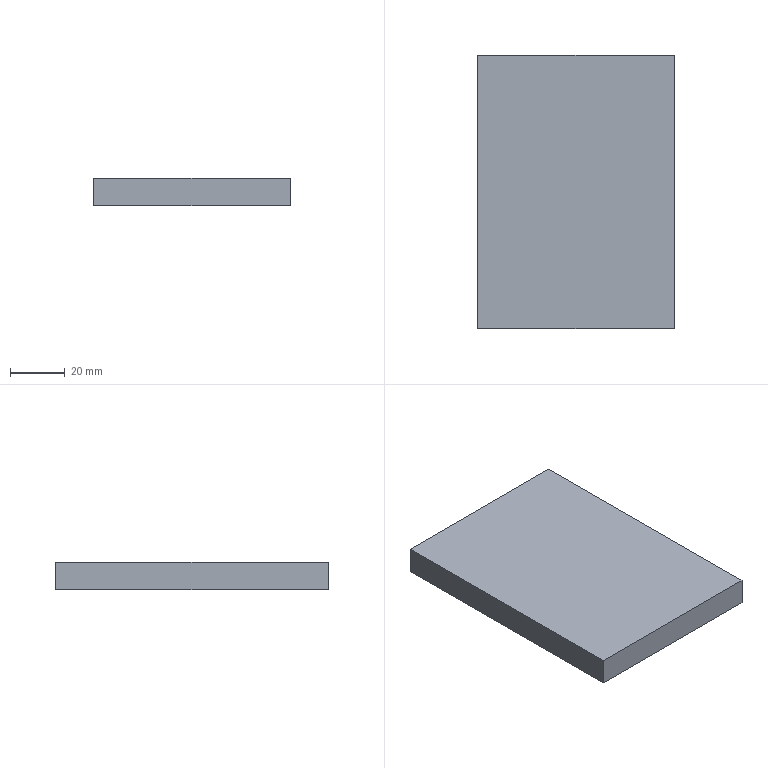Part | STEP file | Display 2 | 1 solid | 6 faces | box 72 x 100 x 10 mm | volume 72000 mm3 | plane 6
STEP:
#1=CARTESIAN_POINT('',(0.,0.,0.));
#2=DIRECTION('',(0.,0.,1.));
#3=DIRECTION('',(1.,0.,0.));
#4=AXIS2_PLACEMENT_3D('',#1,#2,#3);
#5=CARTESIAN_POINT('',(36.,-50.,10.));
#6=VERTEX_POINT('',#5);
#7=CARTESIAN_POINT('',(36.,50.,10.));
#8=VERTEX_POINT('',#7);
#9=CARTESIAN_POINT('',(36.,-50.,10.));
#10=DIRECTION('',(0.,1.,0.));
#11=VECTOR('',#10,1.);
#12=LINE('',#9,#11);
#13=CARTESIAN_POINT('',(-36.,-50.,10.));
#14=DIRECTION('',(0.,0.,1.));
#15=DIRECTION('',(1.,0.,0.));
#16=AXIS2_PLACEMENT_3D('',#13,#14,#15);
#17=PLANE('',#16);
#18=CARTESIAN_POINT('',(72.,0.));
#19=DIRECTION('',(0.,1.));
#20=VECTOR('',#19,1.);
#21=LINE('',#18,#20);
#22=(GEOMETRIC_REPRESENTATION_CONTEXT(2)PARAMETRIC_REPRESENTATION_CONTEXT()REPRESENTATION_CONTEXT('',''));
#23=DEFINITIONAL_REPRESENTATION('',(#21),#22);
#24=PCURVE('',#17,#23);
#25=CARTESIAN_POINT('',(36.,50.,10.));
#26=DIRECTION('',(-1.,0.,0.));
#27=DIRECTION('',(0.,-1.,0.));
#28=AXIS2_PLACEMENT_3D('',#25,#26,#27);
#29=PLANE('',#28);
#30=CARTESIAN_POINT('',(100.,0.));
#31=DIRECTION('',(-1.,0.));
#32=VECTOR('',#31,1.);
#33=LINE('',#30,#32);
#34=(GEOMETRIC_REPRESENTATION_CONTEXT(2)PARAMETRIC_REPRESENTATION_CONTEXT()REPRESENTATION_CONTEXT('',''));
#35=DEFINITIONAL_REPRESENTATION('',(#33),#34);
#36=PCURVE('',#29,#35);
#37=SURFACE_CURVE('',#12,(#24,#36),.PCURVE_S1.);
#38=EDGE_CURVE('',#6,#8,#37,.T.);
#39=ORIENTED_EDGE('',*,*,#38,.T.);
#40=CARTESIAN_POINT('',(-36.,50.,10.));
#41=VERTEX_POINT('',#40);
#42=CARTESIAN_POINT('',(-36.,50.,10.));
#43=DIRECTION('',(-1.,0.,0.));
#44=VECTOR('',#43,1.);
#45=LINE('',#42,#44);
#46=CARTESIAN_POINT('',(0.,100.));
#47=DIRECTION('',(-1.,0.));
#48=VECTOR('',#47,1.);
#49=LINE('',#46,#48);
#50=(GEOMETRIC_REPRESENTATION_CONTEXT(2)PARAMETRIC_REPRESENTATION_CONTEXT()REPRESENTATION_CONTEXT('',''));
#51=DEFINITIONAL_REPRESENTATION('',(#49),#50);
#52=PCURVE('',#17,#51);
#53=CARTESIAN_POINT('',(-36.,50.,10.));
#54=DIRECTION('',(0.,-1.,0.));
#55=DIRECTION('',(1.,0.,0.));
#56=AXIS2_PLACEMENT_3D('',#53,#54,#55);
#57=PLANE('',#56);
#58=CARTESIAN_POINT('',(0.,0.));
#59=DIRECTION('',(-1.,0.));
#60=VECTOR('',#59,1.);
#61=LINE('',#58,#60);
#62=(GEOMETRIC_REPRESENTATION_CONTEXT(2)PARAMETRIC_REPRESENTATION_CONTEXT()REPRESENTATION_CONTEXT('',''));
#63=DEFINITIONAL_REPRESENTATION('',(#61),#62);
#64=PCURVE('',#57,#63);
#65=SURFACE_CURVE('',#45,(#52,#64),.PCURVE_S1.);
#66=EDGE_CURVE('',#8,#41,#65,.T.);
#67=ORIENTED_EDGE('',*,*,#66,.T.);
#68=CARTESIAN_POINT('',(-36.,-50.,10.));
#69=VERTEX_POINT('',#68);
#70=CARTESIAN_POINT('',(-36.,-50.,10.));
#71=DIRECTION('',(0.,-1.,0.));
#72=VECTOR('',#71,1.);
#73=LINE('',#70,#72);
#74=CARTESIAN_POINT('',(0.,0.));
#75=DIRECTION('',(0.,-1.));
#76=VECTOR('',#75,1.);
#77=LINE('',#74,#76);
#78=(GEOMETRIC_REPRESENTATION_CONTEXT(2)PARAMETRIC_REPRESENTATION_CONTEXT()REPRESENTATION_CONTEXT('',''));
#79=DEFINITIONAL_REPRESENTATION('',(#77),#78);
#80=PCURVE('',#17,#79);
#81=CARTESIAN_POINT('',(-36.,50.,10.));
#82=DIRECTION('',(1.,0.,0.));
#83=DIRECTION('',(0.,0.,-1.));
#84=AXIS2_PLACEMENT_3D('',#81,#82,#83);
#85=PLANE('',#84);
#86=CARTESIAN_POINT('',(0.,-100.));
#87=DIRECTION('',(0.,-1.));
#88=VECTOR('',#87,1.);
#89=LINE('',#86,#88);
#90=(GEOMETRIC_REPRESENTATION_CONTEXT(2)PARAMETRIC_REPRESENTATION_CONTEXT()REPRESENTATION_CONTEXT('',''));
#91=DEFINITIONAL_REPRESENTATION('',(#89),#90);
#92=PCURVE('',#85,#91);
#93=SURFACE_CURVE('',#73,(#80,#92),.PCURVE_S1.);
#94=EDGE_CURVE('',#41,#69,#93,.T.);
#95=ORIENTED_EDGE('',*,*,#94,.T.);
#96=CARTESIAN_POINT('',(-36.,-50.,10.));
#97=DIRECTION('',(1.,0.,0.));
#98=VECTOR('',#97,1.);
#99=LINE('',#96,#98);
#100=CARTESIAN_POINT('',(0.,0.));
#101=DIRECTION('',(1.,0.));
#102=VECTOR('',#101,1.);
#103=LINE('',#100,#102);
#104=(GEOMETRIC_REPRESENTATION_CONTEXT(2)PARAMETRIC_REPRESENTATION_CONTEXT()REPRESENTATION_CONTEXT('',''));
#105=DEFINITIONAL_REPRESENTATION('',(#103),#104);
#106=PCURVE('',#17,#105);
#107=CARTESIAN_POINT('',(-36.,-50.,10.));
#108=DIRECTION('',(0.,1.,0.));
#109=DIRECTION('',(-1.,0.,0.));
#110=AXIS2_PLACEMENT_3D('',#107,#108,#109);
#111=PLANE('',#110);
#112=CARTESIAN_POINT('',(0.,0.));
#113=DIRECTION('',(-1.,0.));
#114=VECTOR('',#113,1.);
#115=LINE('',#112,#114);
#116=(GEOMETRIC_REPRESENTATION_CONTEXT(2)PARAMETRIC_REPRESENTATION_CONTEXT()REPRESENTATION_CONTEXT('',''));
#117=DEFINITIONAL_REPRESENTATION('',(#115),#116);
#118=PCURVE('',#111,#117);
#119=SURFACE_CURVE('',#99,(#106,#118),.PCURVE_S1.);
#120=EDGE_CURVE('',#69,#6,#119,.T.);
#121=ORIENTED_EDGE('',*,*,#120,.T.);
#122=EDGE_LOOP('',(#39,#67,#95,#121));
#123=FACE_BOUND('',#122,.T.);
#124=ADVANCED_FACE('',(#123),#17,.T.);
#125=CARTESIAN_POINT('',(-36.,50.,0.));
#126=VERTEX_POINT('',#125);
#127=CARTESIAN_POINT('',(-36.,50.,10.));
#128=DIRECTION('',(0.,0.,-1.));
#129=VECTOR('',#128,1.);
#130=LINE('',#127,#129);
#131=CARTESIAN_POINT('',(0.,0.));
#132=DIRECTION('',(0.,-1.));
#133=VECTOR('',#132,1.);
#134=LINE('',#131,#133);
#135=(GEOMETRIC_REPRESENTATION_CONTEXT(2)PARAMETRIC_REPRESENTATION_CONTEXT()REPRESENTATION_CONTEXT('',''));
#136=DEFINITIONAL_REPRESENTATION('',(#134),#135);
#137=PCURVE('',#57,#136);
#138=CARTESIAN_POINT('',(0.,0.));
#139=DIRECTION('',(1.,0.));
#140=VECTOR('',#139,1.);
#141=LINE('',#138,#140);
#142=(GEOMETRIC_REPRESENTATION_CONTEXT(2)PARAMETRIC_REPRESENTATION_CONTEXT()REPRESENTATION_CONTEXT('',''));
#143=DEFINITIONAL_REPRESENTATION('',(#141),#142);
#144=PCURVE('',#85,#143);
#145=SURFACE_CURVE('',#130,(#137,#144),.PCURVE_S1.);
#146=EDGE_CURVE('',#41,#126,#145,.T.);
#147=ORIENTED_EDGE('',*,*,#146,.F.);
#148=ORIENTED_EDGE('',*,*,#66,.F.);
#149=CARTESIAN_POINT('',(36.,50.,0.));
#150=VERTEX_POINT('',#149);
#151=CARTESIAN_POINT('',(36.,50.,10.));
#152=DIRECTION('',(0.,0.,1.));
#153=VECTOR('',#152,1.);
#154=LINE('',#151,#153);
#155=CARTESIAN_POINT('',(72.,0.));
#156=DIRECTION('',(0.,1.));
#157=VECTOR('',#156,1.);
#158=LINE('',#155,#157);
#159=(GEOMETRIC_REPRESENTATION_CONTEXT(2)PARAMETRIC_REPRESENTATION_CONTEXT()REPRESENTATION_CONTEXT('',''));
#160=DEFINITIONAL_REPRESENTATION('',(#158),#159);
#161=PCURVE('',#57,#160);
#162=CARTESIAN_POINT('',(0.,0.));
#163=DIRECTION('',(0.,1.));
#164=VECTOR('',#163,1.);
#165=LINE('',#162,#164);
#166=(GEOMETRIC_REPRESENTATION_CONTEXT(2)PARAMETRIC_REPRESENTATION_CONTEXT()REPRESENTATION_CONTEXT('',''));
#167=DEFINITIONAL_REPRESENTATION('',(#165),#166);
#168=PCURVE('',#29,#167);
#169=SURFACE_CURVE('',#154,(#161,#168),.PCURVE_S1.);
#170=EDGE_CURVE('',#150,#8,#169,.T.);
#171=ORIENTED_EDGE('',*,*,#170,.F.);
#172=CARTESIAN_POINT('',(-36.,50.,0.));
#173=DIRECTION('',(1.,0.,0.));
#174=VECTOR('',#173,1.);
#175=LINE('',#172,#174);
#176=CARTESIAN_POINT('',(0.,-10.));
#177=DIRECTION('',(1.,0.));
#178=VECTOR('',#177,1.);
#179=LINE('',#176,#178);
#180=(GEOMETRIC_REPRESENTATION_CONTEXT(2)PARAMETRIC_REPRESENTATION_CONTEXT()REPRESENTATION_CONTEXT('',''));
#181=DEFINITIONAL_REPRESENTATION('',(#179),#180);
#182=PCURVE('',#57,#181);
#183=CARTESIAN_POINT('',(-36.,-50.,0.));
#184=DIRECTION('',(0.,0.,1.));
#185=DIRECTION('',(1.,0.,0.));
#186=AXIS2_PLACEMENT_3D('',#183,#184,#185);
#187=PLANE('',#186);
#188=CARTESIAN_POINT('',(0.,100.));
#189=DIRECTION('',(1.,0.));
#190=VECTOR('',#189,1.);
#191=LINE('',#188,#190);
#192=(GEOMETRIC_REPRESENTATION_CONTEXT(2)PARAMETRIC_REPRESENTATION_CONTEXT()REPRESENTATION_CONTEXT('',''));
#193=DEFINITIONAL_REPRESENTATION('',(#191),#192);
#194=PCURVE('',#187,#193);
#195=SURFACE_CURVE('',#175,(#182,#194),.PCURVE_S1.);
#196=EDGE_CURVE('',#126,#150,#195,.T.);
#197=ORIENTED_EDGE('',*,*,#196,.F.);
#198=EDGE_LOOP('',(#147,#148,#171,#197));
#199=FACE_BOUND('',#198,.T.);
#200=ADVANCED_FACE('',(#199),#57,.F.);
#201=ORIENTED_EDGE('',*,*,#170,.T.);
#202=ORIENTED_EDGE('',*,*,#38,.F.);
#203=CARTESIAN_POINT('',(36.,-50.,0.));
#204=VERTEX_POINT('',#203);
#205=CARTESIAN_POINT('',(36.,-50.,10.));
#206=DIRECTION('',(0.,0.,1.));
#207=VECTOR('',#206,1.);
#208=LINE('',#205,#207);
#209=CARTESIAN_POINT('',(100.,0.));
#210=DIRECTION('',(0.,1.));
#211=VECTOR('',#210,1.);
#212=LINE('',#209,#211);
#213=(GEOMETRIC_REPRESENTATION_CONTEXT(2)PARAMETRIC_REPRESENTATION_CONTEXT()REPRESENTATION_CONTEXT('',''));
#214=DEFINITIONAL_REPRESENTATION('',(#212),#213);
#215=PCURVE('',#29,#214);
#216=CARTESIAN_POINT('',(-72.,0.));
#217=DIRECTION('',(0.,1.));
#218=VECTOR('',#217,1.);
#219=LINE('',#216,#218);
#220=(GEOMETRIC_REPRESENTATION_CONTEXT(2)PARAMETRIC_REPRESENTATION_CONTEXT()REPRESENTATION_CONTEXT('',''));
#221=DEFINITIONAL_REPRESENTATION('',(#219),#220);
#222=PCURVE('',#111,#221);
#223=SURFACE_CURVE('',#208,(#215,#222),.PCURVE_S1.);
#224=EDGE_CURVE('',#204,#6,#223,.T.);
#225=ORIENTED_EDGE('',*,*,#224,.F.);
#226=CARTESIAN_POINT('',(36.,50.,0.));
#227=DIRECTION('',(0.,-1.,0.));
#228=VECTOR('',#227,1.);
#229=LINE('',#226,#228);
#230=CARTESIAN_POINT('',(0.,-10.));
#231=DIRECTION('',(1.,0.));
#232=VECTOR('',#231,1.);
#233=LINE('',#230,#232);
#234=(GEOMETRIC_REPRESENTATION_CONTEXT(2)PARAMETRIC_REPRESENTATION_CONTEXT()REPRESENTATION_CONTEXT('',''));
#235=DEFINITIONAL_REPRESENTATION('',(#233),#234);
#236=PCURVE('',#29,#235);
#237=CARTESIAN_POINT('',(72.,100.));
#238=DIRECTION('',(0.,-1.));
#239=VECTOR('',#238,1.);
#240=LINE('',#237,#239);
#241=(GEOMETRIC_REPRESENTATION_CONTEXT(2)PARAMETRIC_REPRESENTATION_CONTEXT()REPRESENTATION_CONTEXT('',''));
#242=DEFINITIONAL_REPRESENTATION('',(#240),#241);
#243=PCURVE('',#187,#242);
#244=SURFACE_CURVE('',#229,(#236,#243),.PCURVE_S1.);
#245=EDGE_CURVE('',#150,#204,#244,.T.);
#246=ORIENTED_EDGE('',*,*,#245,.F.);
#247=EDGE_LOOP('',(#201,#202,#225,#246));
#248=FACE_BOUND('',#247,.T.);
#249=ADVANCED_FACE('',(#248),#29,.F.);
#250=ORIENTED_EDGE('',*,*,#224,.T.);
#251=ORIENTED_EDGE('',*,*,#120,.F.);
#252=CARTESIAN_POINT('',(-36.,-50.,0.));
#253=VERTEX_POINT('',#252);
#254=CARTESIAN_POINT('',(-36.,-50.,10.));
#255=DIRECTION('',(0.,0.,1.));
#256=VECTOR('',#255,1.);
#257=LINE('',#254,#256);
#258=CARTESIAN_POINT('',(0.,0.));
#259=DIRECTION('',(0.,1.));
#260=VECTOR('',#259,1.);
#261=LINE('',#258,#260);
#262=(GEOMETRIC_REPRESENTATION_CONTEXT(2)PARAMETRIC_REPRESENTATION_CONTEXT()REPRESENTATION_CONTEXT('',''));
#263=DEFINITIONAL_REPRESENTATION('',(#261),#262);
#264=PCURVE('',#111,#263);
#265=CARTESIAN_POINT('',(0.,-100.));
#266=DIRECTION('',(-1.,0.));
#267=VECTOR('',#266,1.);
#268=LINE('',#265,#267);
#269=(GEOMETRIC_REPRESENTATION_CONTEXT(2)PARAMETRIC_REPRESENTATION_CONTEXT()REPRESENTATION_CONTEXT('',''));
#270=DEFINITIONAL_REPRESENTATION('',(#268),#269);
#271=PCURVE('',#85,#270);
#272=SURFACE_CURVE('',#257,(#264,#271),.PCURVE_S1.);
#273=EDGE_CURVE('',#253,#69,#272,.T.);
#274=ORIENTED_EDGE('',*,*,#273,.F.);
#275=CARTESIAN_POINT('',(-36.,-50.,0.));
#276=DIRECTION('',(-1.,0.,0.));
#277=VECTOR('',#276,1.);
#278=LINE('',#275,#277);
#279=CARTESIAN_POINT('',(0.,-10.));
#280=DIRECTION('',(1.,0.));
#281=VECTOR('',#280,1.);
#282=LINE('',#279,#281);
#283=(GEOMETRIC_REPRESENTATION_CONTEXT(2)PARAMETRIC_REPRESENTATION_CONTEXT()REPRESENTATION_CONTEXT('',''));
#284=DEFINITIONAL_REPRESENTATION('',(#282),#283);
#285=PCURVE('',#111,#284);
#286=CARTESIAN_POINT('',(0.,0.));
#287=DIRECTION('',(-1.,0.));
#288=VECTOR('',#287,1.);
#289=LINE('',#286,#288);
#290=(GEOMETRIC_REPRESENTATION_CONTEXT(2)PARAMETRIC_REPRESENTATION_CONTEXT()REPRESENTATION_CONTEXT('',''));
#291=DEFINITIONAL_REPRESENTATION('',(#289),#290);
#292=PCURVE('',#187,#291);
#293=SURFACE_CURVE('',#278,(#285,#292),.PCURVE_S1.);
#294=EDGE_CURVE('',#204,#253,#293,.T.);
#295=ORIENTED_EDGE('',*,*,#294,.F.);
#296=EDGE_LOOP('',(#250,#251,#274,#295));
#297=FACE_BOUND('',#296,.T.);
#298=ADVANCED_FACE('',(#297),#111,.F.);
#299=ORIENTED_EDGE('',*,*,#273,.T.);
#300=ORIENTED_EDGE('',*,*,#94,.F.);
#301=ORIENTED_EDGE('',*,*,#146,.T.);
#302=CARTESIAN_POINT('',(-36.,50.,0.));
#303=DIRECTION('',(0.,1.,0.));
#304=VECTOR('',#303,1.);
#305=LINE('',#302,#304);
#306=CARTESIAN_POINT('',(10.,0.));
#307=DIRECTION('',(0.,1.));
#308=VECTOR('',#307,1.);
#309=LINE('',#306,#308);
#310=(GEOMETRIC_REPRESENTATION_CONTEXT(2)PARAMETRIC_REPRESENTATION_CONTEXT()REPRESENTATION_CONTEXT('',''));
#311=DEFINITIONAL_REPRESENTATION('',(#309),#310);
#312=PCURVE('',#85,#311);
#313=CARTESIAN_POINT('',(0.,100.));
#314=DIRECTION('',(0.,1.));
#315=VECTOR('',#314,1.);
#316=LINE('',#313,#315);
#317=(GEOMETRIC_REPRESENTATION_CONTEXT(2)PARAMETRIC_REPRESENTATION_CONTEXT()REPRESENTATION_CONTEXT('',''));
#318=DEFINITIONAL_REPRESENTATION('',(#316),#317);
#319=PCURVE('',#187,#318);
#320=SURFACE_CURVE('',#305,(#312,#319),.PCURVE_S1.);
#321=EDGE_CURVE('',#253,#126,#320,.T.);
#322=ORIENTED_EDGE('',*,*,#321,.F.);
#323=EDGE_LOOP('',(#299,#300,#301,#322));
#324=FACE_BOUND('',#323,.T.);
#325=ADVANCED_FACE('',(#324),#85,.F.);
#326=ORIENTED_EDGE('',*,*,#196,.T.);
#327=ORIENTED_EDGE('',*,*,#245,.T.);
#328=ORIENTED_EDGE('',*,*,#294,.T.);
#329=ORIENTED_EDGE('',*,*,#321,.T.);
#330=EDGE_LOOP('',(#326,#327,#328,#329));
#331=FACE_BOUND('',#330,.T.);
#332=ADVANCED_FACE('',(#331),#187,.F.);
#333=CLOSED_SHELL('',(#124,#200,#249,#298,#325,#332));
#334=MANIFOLD_SOLID_BREP('',#333);
#335=(LENGTH_UNIT()NAMED_UNIT(*)SI_UNIT(.MILLI.,.METRE.));
#336=UNCERTAINTY_MEASURE_WITH_UNIT(LENGTH_MEASURE(0.0000001),#335,'','');
#337=(NAMED_UNIT(*)PLANE_ANGLE_UNIT()SI_UNIT($,.RADIAN.));
#338=(NAMED_UNIT(*)SI_UNIT($,.STERADIAN.)SOLID_ANGLE_UNIT());
#339=(GEOMETRIC_REPRESENTATION_CONTEXT(3)GLOBAL_UNCERTAINTY_ASSIGNED_CONTEXT((#336))GLOBAL_UNIT_ASSIGNED_CONTEXT((#335,#337,#338))REPRESENTATION_CONTEXT('',''));
#340=ADVANCED_BREP_SHAPE_REPRESENTATION('',(#4,#334),#339);